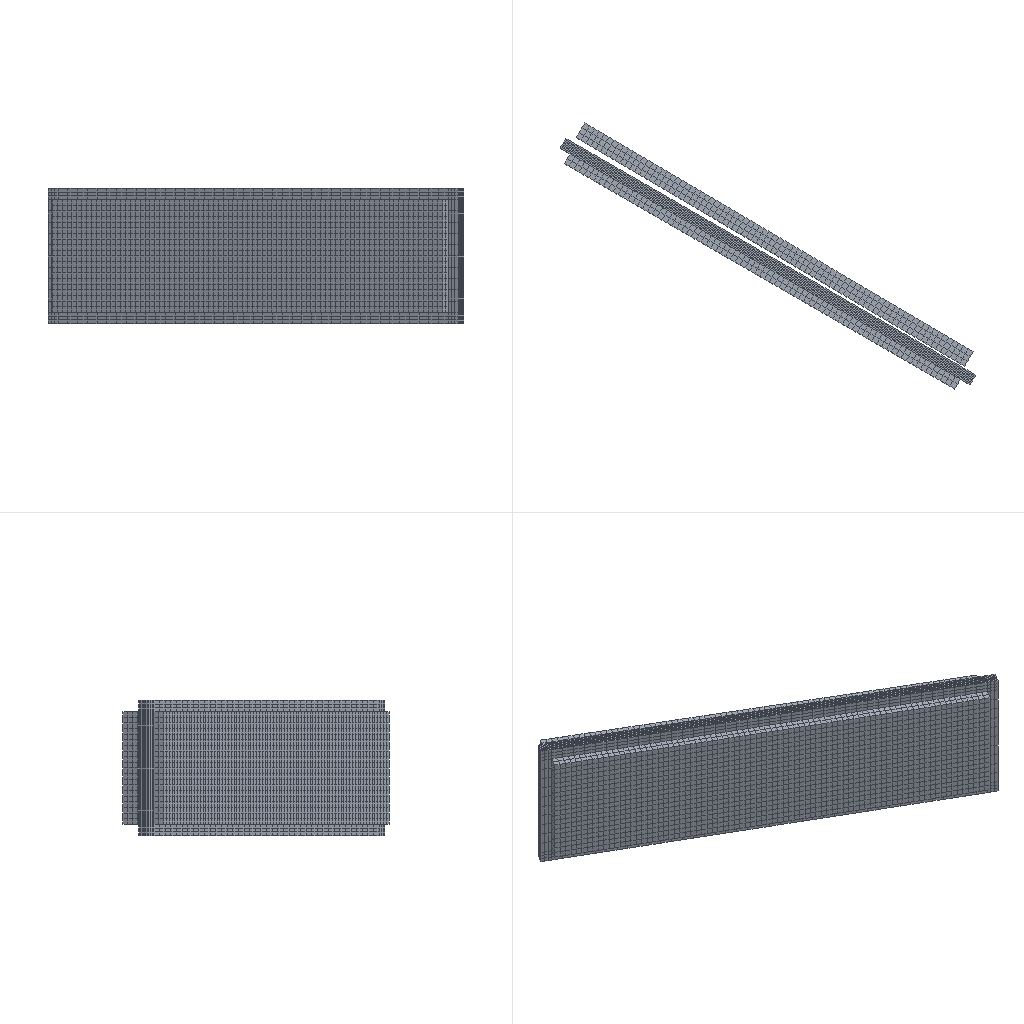Simulation study | abaqus
Set-up summary:
category,name,step,type,value,unit,region
solver,abaqus
solver,version,,,Abaqus/Explicit 2020
units,not stated in the deck,,not stated
analysis,deck,,transient,transient
load_step,Step-1,Step-1,transient
load_step,requested,,,1
mesh,nodes,,,19395
mesh,elements,,,13888
element_type,C3D8R,,solid,9600
element_type,EC3D8R,,solid,4288
load,load commands in deck,,count,1
bc,support commands in deck,,count,13
material,CON,,in results
material,OULA,,in results
check,setup vs results,,match,"per instance, exact: element labels, types and connectivity; labels of the nodes the elements use; coordinates of those nodes at SINGLE_PRECISION in 3 of 3 instance(s)"
Abaqus input file, long lists of numbers shortened:
*Heading
** Job name: Job-2 Model name: Model-1-Copy
** Generated by: Abaqus/CAE 2020
*Preprint, echo=NO, model=NO, history=NO, contact=NO
**
** PARTS
**
*Part, name=coh-oula
*Node
      1,  -40.61,   25.296,    60.782
      2,  -42.342,   26.296,    60.782
** (5785 more lines like these left out)
*Element, type=EC3D8R
  1,    1,   49,  817,   58,   86,  883, 3487,  829
  2,   49,   50,  818,  817,  883,  884, 3488, 3487
** (4286 more lines like these left out)
*Nset, nset=Set-1, generate
    1,  5787,     1
*Elset, elset=Set-1, generate
    1,  4288,     1
** Section: oula
*Eulerian Section, elset=Set-1
oula, oula-1
*Surface, type=EULERIAN MATERIAL, name=oula-1
oula-1
*End Part
**
*Part, name=gaiban
*Node
      1,  -40.508,   26.466,    60.782
      2,  -39.647,   25.958,    60.782
** (6802 more lines like these left out)
*Element, type=C3D8R
   1, 1702, 1703, 1784, 1783,    1,    2,   83,   82
   2, 1703, 1704, 1785, 1784,    2,    3,   84,   83
** (4798 more lines like these left out)
*Nset, nset=Set-1, generate
    1,  6804,     1
*Elset, elset=Set-1, generate
    1,  4800,     1
** Section: wall
*Solid Section, elset=Set-1, material=con
,
*End Part
**
*Part, name=wall
*Node
      1,   28.172,  -15.57,    60.782
      2,   27.306,  -15.07,    60.782
** (6802 more lines like these left out)
*Element, type=C3D8R
   1, 1702, 1703, 1784, 1783,    1,    2,   83,   82
   2, 1703, 1704, 1785, 1784,    2,    3,   84,   83
** (4798 more lines like these left out)
*Nset, nset=Set-1, generate
    1,  6804,     1
*Elset, elset=Set-1, generate
    1,  4800,     1
** Section: wall
*Solid Section, elset=Set-1, material=con
,
*End Part
**
**
** ASSEMBLY
**
*Assembly, name=Assembly
**
*Instance, name=wall-1, part=wall
*End Instance
**
*Instance, name=coh-oula-1, part=coh-oula
*End Instance
**
*Instance, name=gaiban-2, part=gaiban
*End Instance
**
*Nset, nset=Set-1, instance=coh-oula-1
    1,    4,    5,    8,   10,   14,   17,   19,   56,   57,   58,   66,   67,   68,   69,   70
   71,   72,   73,   74,   75,   76,   77,   78,   79,   80,   81,   82,   83,   84,   85,   86
** (139 more lines like these left out)
*Elset, elset=Set-1, instance=coh-oula-1, generate
 1729,  3328,     1
*Nset, nset=Set-2, instance=wall-1, generate
 5104,  6804,     1
*Elset, elset=Set-2, instance=wall-1, generate
 3201,  4800,     1
*Nset, nset=Set-3, instance=coh-oula-1
    2,    3,    6,    7,    9,   12,   13,   16,   18,   20,   21,   22,   23,   24,   25,   26
   27,   29,   30,   31,   32,   33,   34,   35,   36,   37,   38,   40,   41,   42,   43,   44
** (68 more lines like these left out)
*Elset, elset=Set-3, instance=coh-oula-1
    3,    6,    9,   12,   15,   18,   21,   24,   27,   30,   33,   36,   39,   42,   45,   48
   51,   54,   57,   60,   63,   66,   69,   72,   75,   78,   81,   84,   87,   90,   93,   96
** (58 more lines like these left out)
*Nset, nset=Set-5, instance=coh-oula-1
    1,    4,    5,    8,   10,   14,   17,   19,   56,   57,   58,   66,   67,   68,   69,   70
   71,   72,   73,   74,   75,   76,   77,   78,   79,   80,   81,   82,   83,   84,   85,   86
** (139 more lines like these left out)
*Elset, elset=Set-5, instance=coh-oula-1, generate
 1729,  3328,     1
*Nset, nset=Set-7, instance=gaiban-2, generate
 5104,  6804,     1
*Elset, elset=Set-7, instance=gaiban-2, generate
 3201,  4800,     1
*Nset, nset="_T-Datum csys-3", internal
Set-7,
*Transform, nset="_T-Datum csys-3"
0.8616, -0.5075,           0., -0.5075, -0.8616,           0.
*End Assembly
*Amplitude, name=Amp-1
             0.,              0.,           0.001,              1.
**
** MATERIALS
**
*Material, name=con
*Density
 2.8e-09,
*Elastic
28790., 0.22
*Material, name=oula
*Density
 1.1e-09,
*Elastic
 0.8, 0.45
**
** INTERACTION PROPERTIES
**
*Surface Interaction, name=IntProp-1
*Friction
 0.3,
*Surface Behavior, pressure-overclosure=HARD
**
** PREDEFINED FIELDS
**
** Name: Predefined Field-1   Type: Material assignment
*Initial Conditions, type=VOLUME FRACTION
Set-5, coh-oula-1.oula-1, 1.
** ----------------------------------------------------------------
**
** STEP: Step-1
**
*Step, name=Step-1, nlgeom=YES
*Dynamic, Explicit
, 0.001
*Bulk Viscosity
0.06, 1.2
**
** BOUNDARY CONDITIONS
**
** Name: BC-2 Type: 位移/转角
*Boundary
Set-3, 1, 1
Set-3, 2, 2
Set-3, 3, 3
Set-3, 4, 4
Set-3, 5, 5
Set-3, 6, 6
** Name: BC-3 Type: 位移/转角
*Boundary, amplitude=Amp-1
Set-7, 1, 1
Set-7, 2, 2, 1.5
Set-7, 3, 3
Set-7, 4, 4
Set-7, 5, 5
Set-7, 6, 6
** Name: [REDACTED] : Symmetric / antisymmetric / fully fixed
*Boundary
Set-2, ENCASTRE
**
** INTERACTIONS
**
** Interaction: Int-1
*Contact, op=NEW
*Contact Inclusions, ALL EXTERIOR
*Contact Property Assignment
 ,  , IntProp-1
**
** OUTPUT REQUESTS
**
*Restart, write, number interval=1, time marks=NO
**
** FIELD OUTPUT: F-Output-1
**
*Output, field, number interval=40
*Node Output
A, CF, RF, RM, RT, U, V
*Element Output, directions=YES
DENSITYVAVG, E, EVF, LE, MISES, MISESMAX, P, PE, PEEQ, PEEQMAX, PEEQT, PEEQVAVG, PEMAG, PEVAVG, S, SF
SVAVG
*Contact Output
CSTRESS,
**
** HISTORY OUTPUT: H-Output-1
**
*Output, history, variable=PRESELECT
*End Step
Results summary:
result,step,Step-1,completed,increments=5378 time=0.001/0.001
result,analysis,,,transient
result,last_loadstep,,,1
result,primary field,,,U
result,reaction total,,FX,-98.576,model units
result,reaction total,,FY,327.334,model units
result,reaction total,,FZ,-318.065,model units